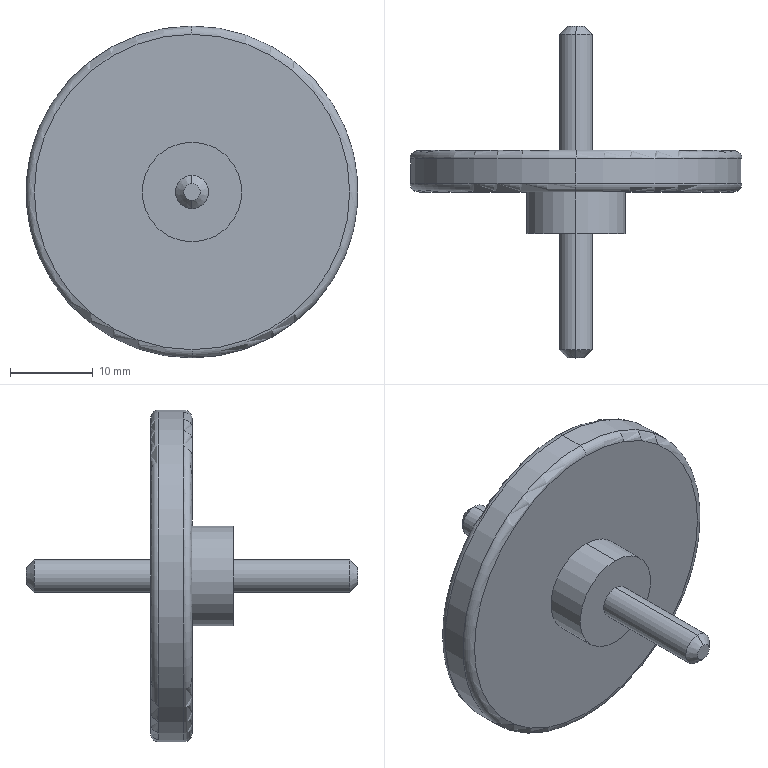Part | SolidWorks | features Chamfer 1, Fillet 1, Revolution 1 | 1 solid | 21 faces | box 40 x 40 x 40 mm | volume 7162 mm3 | cylinder 8 | plane 5 | torus 4 | cone 4 | commonest cylinder face diameters 4 x4 12 x2 40 x2
STEP:
#1=CARTESIAN_POINT('',(0.,25.,19.));
#2=VERTEX_POINT('',#1);
#3=CARTESIAN_POINT('',(0.,25.,-19.));
#4=VERTEX_POINT('',#3);
#5=CARTESIAN_POINT('',(0.,25.,0.));
#6=DIRECTION('',(0.,1.,0.));
#7=DIRECTION('',(0.,0.,-1.));
#8=AXIS2_PLACEMENT_3D('',#5,#6,#7);
#9=CIRCLE('',#8,19.);
#10=EDGE_CURVE('',#2,#4,#9,.T.);
#11=ORIENTED_EDGE('',*,*,#10,.F.);
#12=CARTESIAN_POINT('',(0.,24.,20.));
#13=VERTEX_POINT('',#12);
#14=CARTESIAN_POINT('',(0.,24.,19.));
#15=DIRECTION('',(1.,0.,0.));
#16=DIRECTION('',(0.,1.,0.));
#17=AXIS2_PLACEMENT_3D('',#14,#15,#16);
#18=CIRCLE('',#17,1.);
#19=EDGE_CURVE('',#2,#13,#18,.T.);
#20=ORIENTED_EDGE('',*,*,#19,.T.);
#21=CARTESIAN_POINT('',(0.,24.,-20.));
#22=VERTEX_POINT('',#21);
#23=CARTESIAN_POINT('',(0.,24.,0.));
#24=DIRECTION('',(0.,-1.,0.));
#25=DIRECTION('',(0.,0.,-1.));
#26=AXIS2_PLACEMENT_3D('',#23,#24,#25);
#27=CIRCLE('',#26,20.);
#28=EDGE_CURVE('',#22,#13,#27,.T.);
#29=ORIENTED_EDGE('',*,*,#28,.F.);
#30=CARTESIAN_POINT('',(0.,24.,-19.));
#31=DIRECTION('',(-1.,0.,0.));
#32=DIRECTION('',(0.,-1.,0.));
#33=AXIS2_PLACEMENT_3D('',#30,#31,#32);
#34=CIRCLE('',#33,1.);
#35=EDGE_CURVE('',#4,#22,#34,.T.);
#36=ORIENTED_EDGE('',*,*,#35,.F.);
#37=EDGE_LOOP('',(#11,#20,#29,#36));
#38=FACE_OUTER_BOUND('',#37,.T.);
#39=CARTESIAN_POINT('',(0.,24.,0.));
#40=DIRECTION('',(0.,-1.,0.));
#41=DIRECTION('',(0.,0.,-1.));
#42=AXIS2_PLACEMENT_3D('',#39,#40,#41);
#43=TOROIDAL_SURFACE('',#42,19.,1.);
#44=ADVANCED_FACE('',(#38),#43,.T.);
#45=CARTESIAN_POINT('',(0.,20.,-19.));
#46=VERTEX_POINT('',#45);
#47=CARTESIAN_POINT('',(0.,20.,19.));
#48=VERTEX_POINT('',#47);
#49=CARTESIAN_POINT('',(0.,20.,0.));
#50=DIRECTION('',(0.,-1.,0.));
#51=DIRECTION('',(0.,0.,1.));
#52=AXIS2_PLACEMENT_3D('',#49,#50,#51);
#53=CIRCLE('',#52,19.);
#54=EDGE_CURVE('',#46,#48,#53,.T.);
#55=ORIENTED_EDGE('',*,*,#54,.F.);
#56=CARTESIAN_POINT('',(0.,21.,-20.));
#57=VERTEX_POINT('',#56);
#58=CARTESIAN_POINT('',(0.,21.,-19.));
#59=DIRECTION('',(1.,0.,0.));
#60=DIRECTION('',(0.,1.,0.));
#61=AXIS2_PLACEMENT_3D('',#58,#59,#60);
#62=CIRCLE('',#61,1.);
#63=EDGE_CURVE('',#46,#57,#62,.T.);
#64=ORIENTED_EDGE('',*,*,#63,.T.);
#65=CARTESIAN_POINT('',(0.,21.,20.));
#66=VERTEX_POINT('',#65);
#67=CARTESIAN_POINT('',(0.,21.,0.));
#68=DIRECTION('',(0.,1.,0.));
#69=DIRECTION('',(0.,0.,1.));
#70=AXIS2_PLACEMENT_3D('',#67,#68,#69);
#71=CIRCLE('',#70,20.);
#72=EDGE_CURVE('',#66,#57,#71,.T.);
#73=ORIENTED_EDGE('',*,*,#72,.F.);
#74=CARTESIAN_POINT('',(0.,21.,19.));
#75=DIRECTION('',(-1.,0.,0.));
#76=DIRECTION('',(0.,-1.,0.));
#77=AXIS2_PLACEMENT_3D('',#74,#75,#76);
#78=CIRCLE('',#77,1.);
#79=EDGE_CURVE('',#48,#66,#78,.T.);
#80=ORIENTED_EDGE('',*,*,#79,.F.);
#81=EDGE_LOOP('',(#55,#64,#73,#80));
#82=FACE_OUTER_BOUND('',#81,.T.);
#83=CARTESIAN_POINT('',(0.,21.,0.));
#84=DIRECTION('',(0.,1.,0.));
#85=DIRECTION('',(0.,0.,1.));
#86=AXIS2_PLACEMENT_3D('',#83,#84,#85);
#87=TOROIDAL_SURFACE('',#86,19.,1.);
#88=ADVANCED_FACE('',(#82),#87,.T.);
#89=CARTESIAN_POINT('',(0.,40.,1.));
#90=VERTEX_POINT('',#89);
#91=CARTESIAN_POINT('',(0.,40.,-1.));
#92=VERTEX_POINT('',#91);
#93=CARTESIAN_POINT('',(0.,40.,0.));
#94=DIRECTION('',(0.,1.,0.));
#95=DIRECTION('',(0.,0.,-1.));
#96=AXIS2_PLACEMENT_3D('',#93,#94,#95);
#97=CIRCLE('',#96,1.);
#98=EDGE_CURVE('',#90,#92,#97,.T.);
#99=ORIENTED_EDGE('',*,*,#98,.F.);
#100=CARTESIAN_POINT('',(0.,39.,2.));
#101=VERTEX_POINT('',#100);
#102=CARTESIAN_POINT('',(0.,39.,2.));
#103=DIRECTION('',(0.,-0.7071,0.7071));
#104=VECTOR('',#103,1000.);
#105=LINE('',#102,#104);
#106=EDGE_CURVE('',#90,#101,#105,.T.);
#107=ORIENTED_EDGE('',*,*,#106,.T.);
#108=CARTESIAN_POINT('',(0.,39.,-2.));
#109=VERTEX_POINT('',#108);
#110=CARTESIAN_POINT('',(0.,39.,0.));
#111=DIRECTION('',(0.,-1.,0.));
#112=DIRECTION('',(0.,0.,-1.));
#113=AXIS2_PLACEMENT_3D('',#110,#111,#112);
#114=CIRCLE('',#113,2.);
#115=EDGE_CURVE('',#109,#101,#114,.T.);
#116=ORIENTED_EDGE('',*,*,#115,.F.);
#117=CARTESIAN_POINT('',(0.,39.,-2.));
#118=DIRECTION('',(0.,-0.7071,-0.7071));
#119=VECTOR('',#118,1000.);
#120=LINE('',#117,#119);
#121=EDGE_CURVE('',#92,#109,#120,.T.);
#122=ORIENTED_EDGE('',*,*,#121,.F.);
#123=EDGE_LOOP('',(#99,#107,#116,#122));
#124=FACE_OUTER_BOUND('',#123,.T.);
#125=CARTESIAN_POINT('',(0.,39.,0.));
#126=DIRECTION('',(0.,-1.,0.));
#127=DIRECTION('',(0.,0.,-1.));
#128=AXIS2_PLACEMENT_3D('',#125,#126,#127);
#129=CONICAL_SURFACE('',#128,2.,0.7854);
#130=ADVANCED_FACE('',(#124),#129,.T.);
#131=CARTESIAN_POINT('',(0.,0.,-1.));
#132=VERTEX_POINT('',#131);
#133=CARTESIAN_POINT('',(0.,0.,1.));
#134=VERTEX_POINT('',#133);
#135=CARTESIAN_POINT('',(0.,0.,0.));
#136=DIRECTION('',(0.,-1.,0.));
#137=DIRECTION('',(0.,0.,1.));
#138=AXIS2_PLACEMENT_3D('',#135,#136,#137);
#139=CIRCLE('',#138,1.);
#140=EDGE_CURVE('',#132,#134,#139,.T.);
#141=ORIENTED_EDGE('',*,*,#140,.F.);
#142=CARTESIAN_POINT('',(0.,1.,-2.));
#143=VERTEX_POINT('',#142);
#144=CARTESIAN_POINT('',(0.,0.,-1.));
#145=DIRECTION('',(0.,0.7071,-0.7071));
#146=VECTOR('',#145,1000.);
#147=LINE('',#144,#146);
#148=EDGE_CURVE('',#132,#143,#147,.T.);
#149=ORIENTED_EDGE('',*,*,#148,.T.);
#150=CARTESIAN_POINT('',(0.,1.,2.));
#151=VERTEX_POINT('',#150);
#152=CARTESIAN_POINT('',(0.,1.,0.));
#153=DIRECTION('',(0.,1.,0.));
#154=DIRECTION('',(0.,0.,1.));
#155=AXIS2_PLACEMENT_3D('',#152,#153,#154);
#156=CIRCLE('',#155,2.);
#157=EDGE_CURVE('',#151,#143,#156,.T.);
#158=ORIENTED_EDGE('',*,*,#157,.F.);
#159=CARTESIAN_POINT('',(0.,0.,1.));
#160=DIRECTION('',(0.,0.7071,0.7071));
#161=VECTOR('',#160,1000.);
#162=LINE('',#159,#161);
#163=EDGE_CURVE('',#134,#151,#162,.T.);
#164=ORIENTED_EDGE('',*,*,#163,.F.);
#165=EDGE_LOOP('',(#141,#149,#158,#164));
#166=FACE_OUTER_BOUND('',#165,.T.);
#167=CARTESIAN_POINT('',(0.,0.,0.));
#168=DIRECTION('',(0.,1.,0.));
#169=DIRECTION('',(0.,0.,1.));
#170=AXIS2_PLACEMENT_3D('',#167,#168,#169);
#171=CONICAL_SURFACE('',#170,1.,0.7854);
#172=ADVANCED_FACE('',(#166),#171,.T.);
#173=CARTESIAN_POINT('',(0.,15.,-2.));
#174=VERTEX_POINT('',#173);
#175=CARTESIAN_POINT('',(0.,15.,2.));
#176=VERTEX_POINT('',#175);
#177=CARTESIAN_POINT('',(0.,15.,0.));
#178=DIRECTION('',(0.,-1.,0.));
#179=DIRECTION('',(0.,0.,-1.));
#180=AXIS2_PLACEMENT_3D('',#177,#178,#179);
#181=CIRCLE('',#180,2.);
#182=EDGE_CURVE('',#174,#176,#181,.T.);
#183=ORIENTED_EDGE('',*,*,#182,.T.);
#184=CARTESIAN_POINT('',(0.,0.,2.));
#185=DIRECTION('',(0.,-1.,0.));
#186=VECTOR('',#185,1000.);
#187=LINE('',#184,#186);
#188=EDGE_CURVE('',#176,#151,#187,.T.);
#189=ORIENTED_EDGE('',*,*,#188,.T.);
#190=ORIENTED_EDGE('',*,*,#157,.T.);
#191=CARTESIAN_POINT('',(0.,0.,-2.));
#192=DIRECTION('',(0.,-1.,0.));
#193=VECTOR('',#192,1000.);
#194=LINE('',#191,#193);
#195=EDGE_CURVE('',#174,#143,#194,.T.);
#196=ORIENTED_EDGE('',*,*,#195,.F.);
#197=EDGE_LOOP('',(#183,#189,#190,#196));
#198=FACE_OUTER_BOUND('',#197,.T.);
#199=CARTESIAN_POINT('',(0.,0.,0.));
#200=DIRECTION('',(0.,-1.,0.));
#201=DIRECTION('',(0.,0.,-1.));
#202=AXIS2_PLACEMENT_3D('',#199,#200,#201);
#203=CYLINDRICAL_SURFACE('',#202,2.);
#204=ADVANCED_FACE('',(#198),#203,.T.);
#205=CARTESIAN_POINT('',(0.,20.,-6.));
#206=VERTEX_POINT('',#205);
#207=CARTESIAN_POINT('',(0.,20.,6.));
#208=VERTEX_POINT('',#207);
#209=CARTESIAN_POINT('',(0.,20.,0.));
#210=DIRECTION('',(0.,-1.,0.));
#211=DIRECTION('',(0.,0.,-1.));
#212=AXIS2_PLACEMENT_3D('',#209,#210,#211);
#213=CIRCLE('',#212,6.);
#214=EDGE_CURVE('',#206,#208,#213,.T.);
#215=ORIENTED_EDGE('',*,*,#214,.T.);
#216=CARTESIAN_POINT('',(0.,15.,6.));
#217=VERTEX_POINT('',#216);
#218=CARTESIAN_POINT('',(0.,0.,6.));
#219=DIRECTION('',(0.,-1.,0.));
#220=VECTOR('',#219,1000.);
#221=LINE('',#218,#220);
#222=EDGE_CURVE('',#208,#217,#221,.T.);
#223=ORIENTED_EDGE('',*,*,#222,.T.);
#224=CARTESIAN_POINT('',(0.,15.,-6.));
#225=VERTEX_POINT('',#224);
#226=CARTESIAN_POINT('',(0.,15.,0.));
#227=DIRECTION('',(0.,-1.,0.));
#228=DIRECTION('',(0.,0.,-1.));
#229=AXIS2_PLACEMENT_3D('',#226,#227,#228);
#230=CIRCLE('',#229,6.);
#231=EDGE_CURVE('',#225,#217,#230,.T.);
#232=ORIENTED_EDGE('',*,*,#231,.F.);
#233=CARTESIAN_POINT('',(0.,0.,-6.));
#234=DIRECTION('',(0.,-1.,0.));
#235=VECTOR('',#234,1000.);
#236=LINE('',#233,#235);
#237=EDGE_CURVE('',#206,#225,#236,.T.);
#238=ORIENTED_EDGE('',*,*,#237,.F.);
#239=EDGE_LOOP('',(#215,#223,#232,#238));
#240=FACE_OUTER_BOUND('',#239,.T.);
#241=CARTESIAN_POINT('',(0.,0.,0.));
#242=DIRECTION('',(0.,-1.,0.));
#243=DIRECTION('',(0.,0.,-1.));
#244=AXIS2_PLACEMENT_3D('',#241,#242,#243);
#245=CYLINDRICAL_SURFACE('',#244,6.);
#246=ADVANCED_FACE('',(#240),#245,.T.);
#247=ORIENTED_EDGE('',*,*,#28,.T.);
#248=CARTESIAN_POINT('',(0.,0.,20.));
#249=DIRECTION('',(0.,-1.,0.));
#250=VECTOR('',#249,1000.);
#251=LINE('',#248,#250);
#252=EDGE_CURVE('',#13,#66,#251,.T.);
#253=ORIENTED_EDGE('',*,*,#252,.T.);
#254=ORIENTED_EDGE('',*,*,#72,.T.);
#255=CARTESIAN_POINT('',(0.,0.,-20.));
#256=DIRECTION('',(0.,-1.,0.));
#257=VECTOR('',#256,1000.);
#258=LINE('',#255,#257);
#259=EDGE_CURVE('',#22,#57,#258,.T.);
#260=ORIENTED_EDGE('',*,*,#259,.F.);
#261=EDGE_LOOP('',(#247,#253,#254,#260));
#262=FACE_OUTER_BOUND('',#261,.T.);
#263=CARTESIAN_POINT('',(0.,0.,0.));
#264=DIRECTION('',(0.,-1.,0.));
#265=DIRECTION('',(0.,0.,-1.));
#266=AXIS2_PLACEMENT_3D('',#263,#264,#265);
#267=CYLINDRICAL_SURFACE('',#266,20.);
#268=ADVANCED_FACE('',(#262),#267,.T.);
#269=ORIENTED_EDGE('',*,*,#115,.T.);
#270=CARTESIAN_POINT('',(0.,25.,2.));
#271=VERTEX_POINT('',#270);
#272=CARTESIAN_POINT('',(0.,0.,2.));
#273=DIRECTION('',(0.,-1.,0.));
#274=VECTOR('',#273,1000.);
#275=LINE('',#272,#274);
#276=EDGE_CURVE('',#101,#271,#275,.T.);
#277=ORIENTED_EDGE('',*,*,#276,.T.);
#278=CARTESIAN_POINT('',(0.,25.,-2.));
#279=VERTEX_POINT('',#278);
#280=CARTESIAN_POINT('',(0.,25.,0.));
#281=DIRECTION('',(0.,-1.,0.));
#282=DIRECTION('',(0.,0.,-1.));
#283=AXIS2_PLACEMENT_3D('',#280,#281,#282);
#284=CIRCLE('',#283,2.);
#285=EDGE_CURVE('',#279,#271,#284,.T.);
#286=ORIENTED_EDGE('',*,*,#285,.F.);
#287=CARTESIAN_POINT('',(0.,0.,-2.));
#288=DIRECTION('',(0.,-1.,0.));
#289=VECTOR('',#288,1000.);
#290=LINE('',#287,#289);
#291=EDGE_CURVE('',#109,#279,#290,.T.);
#292=ORIENTED_EDGE('',*,*,#291,.F.);
#293=EDGE_LOOP('',(#269,#277,#286,#292));
#294=FACE_OUTER_BOUND('',#293,.T.);
#295=CARTESIAN_POINT('',(0.,0.,0.));
#296=DIRECTION('',(0.,-1.,0.));
#297=DIRECTION('',(0.,0.,-1.));
#298=AXIS2_PLACEMENT_3D('',#295,#296,#297);
#299=CYLINDRICAL_SURFACE('',#298,2.);
#300=ADVANCED_FACE('',(#294),#299,.T.);
#301=CARTESIAN_POINT('',(0.,40.,0.));
#302=DIRECTION('',(0.,1.,0.));
#303=DIRECTION('',(0.,0.,-1.));
#304=AXIS2_PLACEMENT_3D('',#301,#302,#303);
#305=CIRCLE('',#304,1.);
#306=EDGE_CURVE('',#92,#90,#305,.T.);
#307=ORIENTED_EDGE('',*,*,#306,.T.);
#308=ORIENTED_EDGE('',*,*,#98,.T.);
#309=EDGE_LOOP('',(#307,#308));
#310=FACE_OUTER_BOUND('',#309,.T.);
#311=CARTESIAN_POINT('',(0.,40.,0.));
#312=DIRECTION('',(0.,-1.,0.));
#313=DIRECTION('',(0.,0.,-1.));
#314=AXIS2_PLACEMENT_3D('',#311,#312,#313);
#315=PLANE('',#314);
#316=ADVANCED_FACE('',(#310),#315,.F.);
#317=ORIENTED_EDGE('',*,*,#276,.F.);
#318=CARTESIAN_POINT('',(0.,39.,0.));
#319=DIRECTION('',(0.,-1.,0.));
#320=DIRECTION('',(0.,0.,-1.));
#321=AXIS2_PLACEMENT_3D('',#318,#319,#320);
#322=CIRCLE('',#321,2.);
#323=EDGE_CURVE('',#101,#109,#322,.T.);
#324=ORIENTED_EDGE('',*,*,#323,.T.);
#325=ORIENTED_EDGE('',*,*,#291,.T.);
#326=CARTESIAN_POINT('',(0.,25.,0.));
#327=DIRECTION('',(0.,-1.,0.));
#328=DIRECTION('',(0.,0.,-1.));
#329=AXIS2_PLACEMENT_3D('',#326,#327,#328);
#330=CIRCLE('',#329,2.);
#331=EDGE_CURVE('',#271,#279,#330,.T.);
#332=ORIENTED_EDGE('',*,*,#331,.F.);
#333=EDGE_LOOP('',(#317,#324,#325,#332));
#334=FACE_OUTER_BOUND('',#333,.T.);
#335=CARTESIAN_POINT('',(0.,0.,0.));
#336=DIRECTION('',(0.,-1.,0.));
#337=DIRECTION('',(0.,0.,-1.));
#338=AXIS2_PLACEMENT_3D('',#335,#336,#337);
#339=CYLINDRICAL_SURFACE('',#338,2.);
#340=ADVANCED_FACE('',(#334),#339,.T.);
#341=CARTESIAN_POINT('',(0.,25.,0.));
#342=DIRECTION('',(0.,1.,0.));
#343=DIRECTION('',(0.,0.,-1.));
#344=AXIS2_PLACEMENT_3D('',#341,#342,#343);
#345=CIRCLE('',#344,19.);
#346=EDGE_CURVE('',#4,#2,#345,.T.);
#347=ORIENTED_EDGE('',*,*,#346,.T.);
#348=ORIENTED_EDGE('',*,*,#10,.T.);
#349=EDGE_LOOP('',(#347,#348));
#350=FACE_OUTER_BOUND('',#349,.T.);
#351=ORIENTED_EDGE('',*,*,#285,.T.);
#352=ORIENTED_EDGE('',*,*,#331,.T.);
#353=EDGE_LOOP('',(#351,#352));
#354=FACE_BOUND('',#353,.T.);
#355=CARTESIAN_POINT('',(-2.,25.,0.));
#356=DIRECTION('',(0.,-1.,0.));
#357=DIRECTION('',(0.,0.,-1.));
#358=AXIS2_PLACEMENT_3D('',#355,#356,#357);
#359=PLANE('',#358);
#360=ADVANCED_FACE('',(#350,#354),#359,.F.);
#361=ORIENTED_EDGE('',*,*,#252,.F.);
#362=CARTESIAN_POINT('',(0.,24.,0.));
#363=DIRECTION('',(0.,-1.,0.));
#364=DIRECTION('',(0.,0.,-1.));
#365=AXIS2_PLACEMENT_3D('',#362,#363,#364);
#366=CIRCLE('',#365,20.);
#367=EDGE_CURVE('',#13,#22,#366,.T.);
#368=ORIENTED_EDGE('',*,*,#367,.T.);
#369=ORIENTED_EDGE('',*,*,#259,.T.);
#370=CARTESIAN_POINT('',(0.,21.,0.));
#371=DIRECTION('',(0.,1.,0.));
#372=DIRECTION('',(0.,0.,1.));
#373=AXIS2_PLACEMENT_3D('',#370,#371,#372);
#374=CIRCLE('',#373,20.);
#375=EDGE_CURVE('',#57,#66,#374,.T.);
#376=ORIENTED_EDGE('',*,*,#375,.T.);
#377=EDGE_LOOP('',(#361,#368,#369,#376));
#378=FACE_OUTER_BOUND('',#377,.T.);
#379=CARTESIAN_POINT('',(0.,0.,0.));
#380=DIRECTION('',(0.,-1.,0.));
#381=DIRECTION('',(0.,0.,-1.));
#382=AXIS2_PLACEMENT_3D('',#379,#380,#381);
#383=CYLINDRICAL_SURFACE('',#382,20.);
#384=ADVANCED_FACE('',(#378),#383,.T.);
#385=CARTESIAN_POINT('',(0.,20.,0.));
#386=DIRECTION('',(0.,-1.,0.));
#387=DIRECTION('',(0.,0.,1.));
#388=AXIS2_PLACEMENT_3D('',#385,#386,#387);
#389=CIRCLE('',#388,19.);
#390=EDGE_CURVE('',#48,#46,#389,.T.);
#391=ORIENTED_EDGE('',*,*,#390,.T.);
#392=ORIENTED_EDGE('',*,*,#54,.T.);
#393=EDGE_LOOP('',(#391,#392));
#394=FACE_OUTER_BOUND('',#393,.T.);
#395=ORIENTED_EDGE('',*,*,#214,.F.);
#396=CARTESIAN_POINT('',(0.,20.,0.));
#397=DIRECTION('',(0.,-1.,0.));
#398=DIRECTION('',(0.,0.,-1.));
#399=AXIS2_PLACEMENT_3D('',#396,#397,#398);
#400=CIRCLE('',#399,6.);
#401=EDGE_CURVE('',#208,#206,#400,.T.);
#402=ORIENTED_EDGE('',*,*,#401,.F.);
#403=EDGE_LOOP('',(#395,#402));
#404=FACE_BOUND('',#403,.T.);
#405=CARTESIAN_POINT('',(-20.,20.,0.));
#406=DIRECTION('',(0.,1.,0.));
#407=DIRECTION('',(0.,0.,1.));
#408=AXIS2_PLACEMENT_3D('',#405,#406,#407);
#409=PLANE('',#408);
#410=ADVANCED_FACE('',(#394,#404),#409,.F.);
#411=ORIENTED_EDGE('',*,*,#222,.F.);
#412=ORIENTED_EDGE('',*,*,#401,.T.);
#413=ORIENTED_EDGE('',*,*,#237,.T.);
#414=CARTESIAN_POINT('',(0.,15.,0.));
#415=DIRECTION('',(0.,-1.,0.));
#416=DIRECTION('',(0.,0.,-1.));
#417=AXIS2_PLACEMENT_3D('',#414,#415,#416);
#418=CIRCLE('',#417,6.);
#419=EDGE_CURVE('',#217,#225,#418,.T.);
#420=ORIENTED_EDGE('',*,*,#419,.F.);
#421=EDGE_LOOP('',(#411,#412,#413,#420));
#422=FACE_OUTER_BOUND('',#421,.T.);
#423=CARTESIAN_POINT('',(0.,0.,0.));
#424=DIRECTION('',(0.,-1.,0.));
#425=DIRECTION('',(0.,0.,-1.));
#426=AXIS2_PLACEMENT_3D('',#423,#424,#425);
#427=CYLINDRICAL_SURFACE('',#426,6.);
#428=ADVANCED_FACE('',(#422),#427,.T.);
#429=ORIENTED_EDGE('',*,*,#182,.F.);
#430=CARTESIAN_POINT('',(0.,15.,0.));
#431=DIRECTION('',(0.,-1.,0.));
#432=DIRECTION('',(0.,0.,-1.));
#433=AXIS2_PLACEMENT_3D('',#430,#431,#432);
#434=CIRCLE('',#433,2.);
#435=EDGE_CURVE('',#176,#174,#434,.T.);
#436=ORIENTED_EDGE('',*,*,#435,.F.);
#437=EDGE_LOOP('',(#429,#436));
#438=FACE_BOUND('',#437,.T.);
#439=ORIENTED_EDGE('',*,*,#231,.T.);
#440=ORIENTED_EDGE('',*,*,#419,.T.);
#441=EDGE_LOOP('',(#439,#440));
#442=FACE_OUTER_BOUND('',#441,.T.);
#443=CARTESIAN_POINT('',(-6.,15.,0.));
#444=DIRECTION('',(0.,1.,0.));
#445=DIRECTION('',(0.,0.,1.));
#446=AXIS2_PLACEMENT_3D('',#443,#444,#445);
#447=PLANE('',#446);
#448=ADVANCED_FACE('',(#438,#442),#447,.F.);
#449=ORIENTED_EDGE('',*,*,#188,.F.);
#450=ORIENTED_EDGE('',*,*,#435,.T.);
#451=ORIENTED_EDGE('',*,*,#195,.T.);
#452=CARTESIAN_POINT('',(0.,1.,0.));
#453=DIRECTION('',(0.,1.,0.));
#454=DIRECTION('',(0.,0.,1.));
#455=AXIS2_PLACEMENT_3D('',#452,#453,#454);
#456=CIRCLE('',#455,2.);
#457=EDGE_CURVE('',#143,#151,#456,.T.);
#458=ORIENTED_EDGE('',*,*,#457,.T.);
#459=EDGE_LOOP('',(#449,#450,#451,#458));
#460=FACE_OUTER_BOUND('',#459,.T.);
#461=CARTESIAN_POINT('',(0.,0.,0.));
#462=DIRECTION('',(0.,-1.,0.));
#463=DIRECTION('',(0.,0.,-1.));
#464=AXIS2_PLACEMENT_3D('',#461,#462,#463);
#465=CYLINDRICAL_SURFACE('',#464,2.);
#466=ADVANCED_FACE('',(#460),#465,.T.);
#467=CARTESIAN_POINT('',(0.,0.,0.));
#468=DIRECTION('',(0.,-1.,0.));
#469=DIRECTION('',(0.,0.,1.));
#470=AXIS2_PLACEMENT_3D('',#467,#468,#469);
#471=CIRCLE('',#470,1.);
#472=EDGE_CURVE('',#134,#132,#471,.T.);
#473=ORIENTED_EDGE('',*,*,#472,.T.);
#474=ORIENTED_EDGE('',*,*,#140,.T.);
#475=EDGE_LOOP('',(#473,#474));
#476=FACE_OUTER_BOUND('',#475,.T.);
#477=CARTESIAN_POINT('',(-2.,0.,0.));
#478=DIRECTION('',(0.,1.,0.));
#479=DIRECTION('',(0.,0.,1.));
#480=AXIS2_PLACEMENT_3D('',#477,#478,#479);
#481=PLANE('',#480);
#482=ADVANCED_FACE('',(#476),#481,.F.);
#483=ORIENTED_EDGE('',*,*,#148,.F.);
#484=ORIENTED_EDGE('',*,*,#472,.F.);
#485=ORIENTED_EDGE('',*,*,#163,.T.);
#486=ORIENTED_EDGE('',*,*,#457,.F.);
#487=EDGE_LOOP('',(#483,#484,#485,#486));
#488=FACE_OUTER_BOUND('',#487,.T.);
#489=CARTESIAN_POINT('',(0.,0.,0.));
#490=DIRECTION('',(0.,1.,0.));
#491=DIRECTION('',(0.,0.,1.));
#492=AXIS2_PLACEMENT_3D('',#489,#490,#491);
#493=CONICAL_SURFACE('',#492,1.,0.7854);
#494=ADVANCED_FACE('',(#488),#493,.T.);
#495=ORIENTED_EDGE('',*,*,#106,.F.);
#496=ORIENTED_EDGE('',*,*,#306,.F.);
#497=ORIENTED_EDGE('',*,*,#121,.T.);
#498=ORIENTED_EDGE('',*,*,#323,.F.);
#499=EDGE_LOOP('',(#495,#496,#497,#498));
#500=FACE_OUTER_BOUND('',#499,.T.);
#501=CARTESIAN_POINT('',(0.,39.,0.));
#502=DIRECTION('',(0.,-1.,0.));
#503=DIRECTION('',(0.,0.,-1.));
#504=AXIS2_PLACEMENT_3D('',#501,#502,#503);
#505=CONICAL_SURFACE('',#504,2.,0.7854);
#506=ADVANCED_FACE('',(#500),#505,.T.);
#507=ORIENTED_EDGE('',*,*,#63,.F.);
#508=ORIENTED_EDGE('',*,*,#390,.F.);
#509=ORIENTED_EDGE('',*,*,#79,.T.);
#510=ORIENTED_EDGE('',*,*,#375,.F.);
#511=EDGE_LOOP('',(#507,#508,#509,#510));
#512=FACE_OUTER_BOUND('',#511,.T.);
#513=CARTESIAN_POINT('',(0.,21.,0.));
#514=DIRECTION('',(0.,1.,0.));
#515=DIRECTION('',(0.,0.,1.));
#516=AXIS2_PLACEMENT_3D('',#513,#514,#515);
#517=TOROIDAL_SURFACE('',#516,19.,1.);
#518=ADVANCED_FACE('',(#512),#517,.T.);
#519=ORIENTED_EDGE('',*,*,#19,.F.);
#520=ORIENTED_EDGE('',*,*,#346,.F.);
#521=ORIENTED_EDGE('',*,*,#35,.T.);
#522=ORIENTED_EDGE('',*,*,#367,.F.);
#523=EDGE_LOOP('',(#519,#520,#521,#522));
#524=FACE_OUTER_BOUND('',#523,.T.);
#525=CARTESIAN_POINT('',(0.,24.,0.));
#526=DIRECTION('',(0.,-1.,0.));
#527=DIRECTION('',(0.,0.,-1.));
#528=AXIS2_PLACEMENT_3D('',#525,#526,#527);
#529=TOROIDAL_SURFACE('',#528,19.,1.);
#530=ADVANCED_FACE('',(#524),#529,.T.);
#531=CLOSED_SHELL('',(#44,#88,#130,#172,#204,#246,#268,#300,#316,#340,#360,#384,#410,#428,#448,#466,#482,#494,#506,#518,#530));
#532=MANIFOLD_SOLID_BREP('',#531);
#533=CARTESIAN_POINT('',(0.,0.,0.));
#534=DIRECTION('',(0.,0.,1.));
#535=DIRECTION('',(1.,0.,0.));
#536=AXIS2_PLACEMENT_3D('',#533,#534,#535);
#537=(LENGTH_UNIT()NAMED_UNIT(*)SI_UNIT(.MILLI.,.METRE.));
#538=UNCERTAINTY_MEASURE_WITH_UNIT(LENGTH_MEASURE(0.00001),#537,'','');
#539=(NAMED_UNIT(*)PLANE_ANGLE_UNIT()SI_UNIT($,.RADIAN.));
#540=(NAMED_UNIT(*)SI_UNIT($,.STERADIAN.)SOLID_ANGLE_UNIT());
#541=(GEOMETRIC_REPRESENTATION_CONTEXT(3)GLOBAL_UNCERTAINTY_ASSIGNED_CONTEXT((#538))GLOBAL_UNIT_ASSIGNED_CONTEXT((#537,#539,#540))REPRESENTATION_CONTEXT('',''));
#542=ADVANCED_BREP_SHAPE_REPRESENTATION('',(#532,#536),#541);